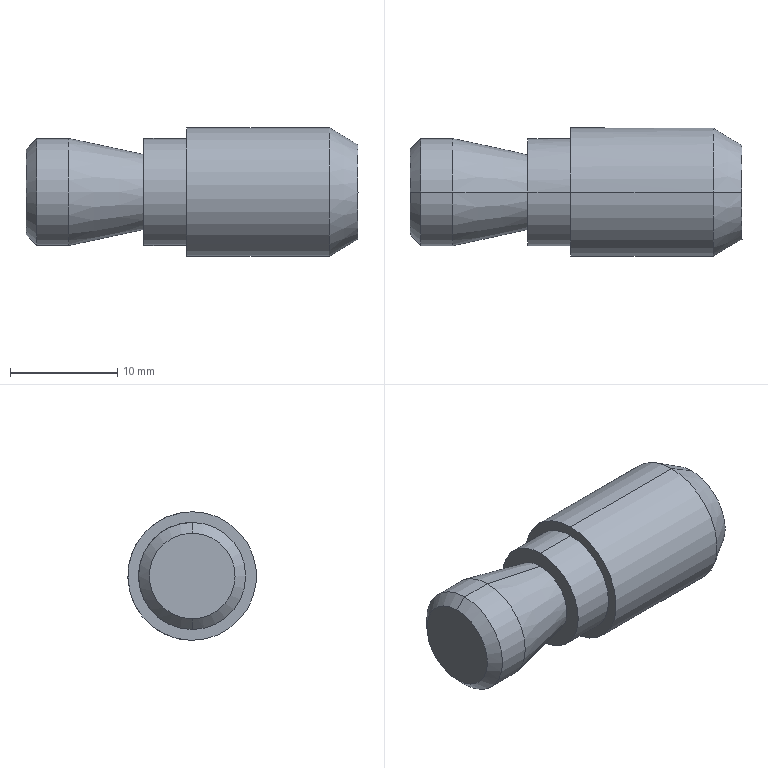Part | STEP file | Positioning_id2322_x_t | 1 solid | 16 faces | box 31 x 12 x 12 mm | volume 2751 mm3 | cone 6 | cylinder 6 | plane 4 | commonest cylinder face diameters 10 x4 12 x2
STEP:
#1=CARTESIAN_POINT('',(0.,0.,0.));
#2=DIRECTION('',(0.,0.,1.));
#3=DIRECTION('',(1.,0.,0.));
#4=AXIS2_PLACEMENT_3D('',#1,#2,#3);
#5=CARTESIAN_POINT('',(-648.,468.,127.399));
#6=VERTEX_POINT('',#5);
#7=CARTESIAN_POINT('',(-650.667,468.,128.999));
#8=VERTEX_POINT('',#7);
#9=CARTESIAN_POINT('',(-648.,468.,127.399));
#10=DIRECTION('',(-0.8575,0.,0.5145));
#11=VECTOR('',#10,1.);
#12=LINE('',#9,#11);
#13=CARTESIAN_POINT('',(-654.,468.,122.999));
#14=DIRECTION('',(-1.,0.,0.));
#15=DIRECTION('',(0.,0.,1.));
#16=AXIS2_PLACEMENT_3D('',#13,#14,#15);
#17=CONICAL_SURFACE('',#16,8.,0.5404);
#18=CARTESIAN_POINT('',(0.,-6.));
#19=DIRECTION('',(0.,1.));
#20=VECTOR('',#19,1.);
#21=LINE('',#18,#20);
#22=(GEOMETRIC_REPRESENTATION_CONTEXT(2)PARAMETRIC_REPRESENTATION_CONTEXT()REPRESENTATION_CONTEXT('',''));
#23=DEFINITIONAL_REPRESENTATION('',(#21),#22);
#24=PCURVE('',#17,#23);
#25=CARTESIAN_POINT('',(-654.,468.,122.999));
#26=DIRECTION('',(-1.,0.,0.));
#27=DIRECTION('',(0.,0.,1.));
#28=AXIS2_PLACEMENT_3D('',#25,#26,#27);
#29=CONICAL_SURFACE('',#28,8.,0.5404);
#30=CARTESIAN_POINT('',(6.283,-6.));
#31=DIRECTION('',(0.,1.));
#32=VECTOR('',#31,1.);
#33=LINE('',#30,#32);
#34=(GEOMETRIC_REPRESENTATION_CONTEXT(2)PARAMETRIC_REPRESENTATION_CONTEXT()REPRESENTATION_CONTEXT('',''));
#35=DEFINITIONAL_REPRESENTATION('',(#33),#34);
#36=PCURVE('',#29,#35);
#37=SURFACE_CURVE('',#12,(#24,#36),.PCURVE_S1.);
#38=EDGE_CURVE('',#6,#8,#37,.T.);
#39=ORIENTED_EDGE('',*,*,#38,.F.);
#40=CARTESIAN_POINT('',(-648.,468.,118.599));
#41=VERTEX_POINT('',#40);
#42=CARTESIAN_POINT('',(-648.,468.,122.999));
#43=DIRECTION('',(-1.,0.,0.));
#44=DIRECTION('',(0.,0.,1.));
#45=AXIS2_PLACEMENT_3D('',#42,#43,#44);
#46=CIRCLE('',#45,4.4);
#47=CARTESIAN_POINT('',(0.,-6.));
#48=DIRECTION('',(1.,0.));
#49=VECTOR('',#48,1.);
#50=LINE('',#47,#49);
#51=(GEOMETRIC_REPRESENTATION_CONTEXT(2)PARAMETRIC_REPRESENTATION_CONTEXT()REPRESENTATION_CONTEXT('',''));
#52=DEFINITIONAL_REPRESENTATION('',(#50),#51);
#53=PCURVE('',#17,#52);
#54=CARTESIAN_POINT('',(-648.,468.,122.999));
#55=DIRECTION('',(1.,0.,0.));
#56=DIRECTION('',(0.,0.,1.));
#57=AXIS2_PLACEMENT_3D('',#54,#55,#56);
#58=PLANE('',#57);
#59=CARTESIAN_POINT('',(4.4,0.));
#60=CARTESIAN_POINT('',(4.4,-7.621));
#61=CARTESIAN_POINT('',(-2.2,-3.811));
#62=CARTESIAN_POINT('',(-8.8,0.));
#63=CARTESIAN_POINT('',(-2.2,3.811));
#64=CARTESIAN_POINT('',(4.4,7.621));
#65=CARTESIAN_POINT('',(4.4,0.));
#66=(BOUNDED_CURVE()B_SPLINE_CURVE(2,(#59,#60,#61,#62,#63,#64,#65),.UNSPECIFIED.,.T.,.F.)B_SPLINE_CURVE_WITH_KNOTS((1,2,2,2,2,1),(-2.094,0.,2.094,4.189,6.283,8.378),.UNSPECIFIED.)CURVE()GEOMETRIC_REPRESENTATION_ITEM()RATIONAL_B_SPLINE_CURVE((1.,0.5,1.,0.5,1.,0.5,1.))REPRESENTATION_ITEM(''));
#67=(GEOMETRIC_REPRESENTATION_CONTEXT(2)PARAMETRIC_REPRESENTATION_CONTEXT()REPRESENTATION_CONTEXT('',''));
#68=DEFINITIONAL_REPRESENTATION('',(#66),#67);
#69=PCURVE('',#58,#68);
#70=SURFACE_CURVE('',#46,(#53,#69),.PCURVE_S1.);
#71=EDGE_CURVE('',#6,#41,#70,.T.);
#72=ORIENTED_EDGE('',*,*,#71,.T.);
#73=CARTESIAN_POINT('',(-650.667,468.,116.999));
#74=VERTEX_POINT('',#73);
#75=CARTESIAN_POINT('',(-648.,468.,118.599));
#76=DIRECTION('',(0.8575,0.,0.5145));
#77=VECTOR('',#76,1.);
#78=LINE('',#75,#77);
#79=CARTESIAN_POINT('',(3.142,-6.));
#80=DIRECTION('',(0.,-1.));
#81=VECTOR('',#80,1.);
#82=LINE('',#79,#81);
#83=(GEOMETRIC_REPRESENTATION_CONTEXT(2)PARAMETRIC_REPRESENTATION_CONTEXT()REPRESENTATION_CONTEXT('',''));
#84=DEFINITIONAL_REPRESENTATION('',(#82),#83);
#85=PCURVE('',#17,#84);
#86=CARTESIAN_POINT('',(3.142,-6.));
#87=DIRECTION('',(0.,-1.));
#88=VECTOR('',#87,1.);
#89=LINE('',#86,#88);
#90=(GEOMETRIC_REPRESENTATION_CONTEXT(2)PARAMETRIC_REPRESENTATION_CONTEXT()REPRESENTATION_CONTEXT('',''));
#91=DEFINITIONAL_REPRESENTATION('',(#89),#90);
#92=PCURVE('',#29,#91);
#93=SURFACE_CURVE('',#78,(#85,#92),.PCURVE_S1.);
#94=EDGE_CURVE('',#74,#41,#93,.T.);
#95=ORIENTED_EDGE('',*,*,#94,.F.);
#96=CARTESIAN_POINT('',(-650.667,468.,122.999));
#97=DIRECTION('',(1.,0.,0.));
#98=DIRECTION('',(0.,0.,-1.));
#99=AXIS2_PLACEMENT_3D('',#96,#97,#98);
#100=CIRCLE('',#99,6.);
#101=CARTESIAN_POINT('',(3.142,-3.333));
#102=DIRECTION('',(-1.,0.));
#103=VECTOR('',#102,1.);
#104=LINE('',#101,#103);
#105=(GEOMETRIC_REPRESENTATION_CONTEXT(2)PARAMETRIC_REPRESENTATION_CONTEXT()REPRESENTATION_CONTEXT('',''));
#106=DEFINITIONAL_REPRESENTATION('',(#104),#105);
#107=PCURVE('',#17,#106);
#108=CARTESIAN_POINT('',(-669.,468.,122.999));
#109=DIRECTION('',(-1.,0.,0.));
#110=DIRECTION('',(0.,0.,1.));
#111=AXIS2_PLACEMENT_3D('',#108,#109,#110);
#112=CYLINDRICAL_SURFACE('',#111,6.);
#113=CARTESIAN_POINT('',(3.142,-18.333));
#114=DIRECTION('',(-1.,0.));
#115=VECTOR('',#114,1.);
#116=LINE('',#113,#115);
#117=(GEOMETRIC_REPRESENTATION_CONTEXT(2)PARAMETRIC_REPRESENTATION_CONTEXT()REPRESENTATION_CONTEXT('',''));
#118=DEFINITIONAL_REPRESENTATION('',(#116),#117);
#119=PCURVE('',#112,#118);
#120=SURFACE_CURVE('',#100,(#107,#119),.PCURVE_S1.);
#121=EDGE_CURVE('',#74,#8,#120,.T.);
#122=ORIENTED_EDGE('',*,*,#121,.T.);
#123=EDGE_LOOP('',(#39,#72,#95,#122));
#124=FACE_BOUND('',#123,.T.);
#125=ADVANCED_FACE('',(#124),#17,.T.);
#126=CARTESIAN_POINT('',(-648.,468.,118.599));
#127=CARTESIAN_POINT('',(-648.,463.6,118.599));
#128=CARTESIAN_POINT('',(-648.,461.4,122.999));
#129=CARTESIAN_POINT('',(-648.,463.6,127.399));
#130=CARTESIAN_POINT('',(-648.,468.,127.399));
#131=(BOUNDED_CURVE()B_SPLINE_CURVE(4,(#126,#127,#128,#129,#130),.UNSPECIFIED.,.F.,.F.)B_SPLINE_CURVE_WITH_KNOTS((5,5),(0.,1.),.PIECEWISE_BEZIER_KNOTS.)CURVE()GEOMETRIC_REPRESENTATION_ITEM()RATIONAL_B_SPLINE_CURVE((1.,0.7071,0.6667,0.7071,1.))REPRESENTATION_ITEM(''));
#132=CARTESIAN_POINT('',(-4.4,0.));
#133=CARTESIAN_POINT('',(-4.4,4.4));
#134=CARTESIAN_POINT('',(0.,6.6));
#135=CARTESIAN_POINT('',(4.4,4.4));
#136=CARTESIAN_POINT('',(4.4,0.));
#137=(BOUNDED_CURVE()B_SPLINE_CURVE(4,(#132,#133,#134,#135,#136),.UNSPECIFIED.,.F.,.F.)B_SPLINE_CURVE_WITH_KNOTS((5,5),(0.,1.),.PIECEWISE_BEZIER_KNOTS.)CURVE()GEOMETRIC_REPRESENTATION_ITEM()RATIONAL_B_SPLINE_CURVE((1.,0.7071,0.6667,0.7071,1.))REPRESENTATION_ITEM(''));
#138=(GEOMETRIC_REPRESENTATION_CONTEXT(2)PARAMETRIC_REPRESENTATION_CONTEXT()REPRESENTATION_CONTEXT('',''));
#139=DEFINITIONAL_REPRESENTATION('',(#137),#138);
#140=PCURVE('',#58,#139);
#141=CARTESIAN_POINT('',(3.142,-6.));
#142=CARTESIAN_POINT('',(3.184,-6.));
#143=CARTESIAN_POINT('',(3.271,-6.));
#144=CARTESIAN_POINT('',(3.405,-6.));
#145=CARTESIAN_POINT('',(3.542,-6.));
#146=CARTESIAN_POINT('',(3.681,-6.));
#147=CARTESIAN_POINT('',(3.823,-6.));
#148=CARTESIAN_POINT('',(3.968,-6.));
#149=CARTESIAN_POINT('',(4.114,-6.));
#150=CARTESIAN_POINT('',(4.262,-6.));
#151=CARTESIAN_POINT('',(4.412,-6.));
#152=CARTESIAN_POINT('',(4.562,-6.));
#153=CARTESIAN_POINT('',(4.712,-6.));
#154=CARTESIAN_POINT('',(4.863,-6.));
#155=CARTESIAN_POINT('',(5.013,-6.));
#156=CARTESIAN_POINT('',(5.163,-6.));
#157=CARTESIAN_POINT('',(5.311,-6.));
#158=CARTESIAN_POINT('',(5.457,-6.));
#159=CARTESIAN_POINT('',(5.602,-6.));
#160=CARTESIAN_POINT('',(5.744,-6.));
#161=CARTESIAN_POINT('',(5.883,-6.));
#162=CARTESIAN_POINT('',(6.02,-6.));
#163=CARTESIAN_POINT('',(6.153,-6.));
#164=CARTESIAN_POINT('',(6.24,-6.));
#165=CARTESIAN_POINT('',(6.283,-6.));
#166=B_SPLINE_CURVE_WITH_KNOTS('',3,(#141,#142,#143,#144,#145,#146,#147,#148,#149,#150,#151,#152,#153,#154,#155,#156,#157,#158,#159,#160,#161,#162,#163,#164,#165),.UNSPECIFIED.,.F.,.F.,(4,1,1,1,1,1,1,1,1,1,1,1,1,1,1,1,1,1,1,1,1,1,4),(0.,0.04545,0.09091,0.1364,0.1818,0.2273,0.2727,0.3182,0.3636,0.4091,0.4545,0.5,0.5455,0.5909,0.6364,0.6818,0.7273,0.7727,0.8182,0.8636,0.9091,0.9545,1.),.QUASI_UNIFORM_KNOTS.);
#167=(GEOMETRIC_REPRESENTATION_CONTEXT(2)PARAMETRIC_REPRESENTATION_CONTEXT()REPRESENTATION_CONTEXT('',''));
#168=DEFINITIONAL_REPRESENTATION('',(#166),#167);
#169=PCURVE('',#29,#168);
#170=SURFACE_CURVE('',#131,(#140,#169),.PCURVE_S1.);
#171=EDGE_CURVE('',#41,#6,#170,.T.);
#172=ORIENTED_EDGE('',*,*,#171,.F.);
#173=ORIENTED_EDGE('',*,*,#71,.F.);
#174=EDGE_LOOP('',(#172,#173));
#175=FACE_BOUND('',#174,.T.);
#176=ADVANCED_FACE('',(#175),#58,.T.);
#177=CARTESIAN_POINT('',(-668.,468.,119.499));
#178=VERTEX_POINT('',#177);
#179=CARTESIAN_POINT('',(-668.,468.,126.499));
#180=VERTEX_POINT('',#179);
#181=CARTESIAN_POINT('',(-668.,468.,122.999));
#182=DIRECTION('',(-1.,0.,0.));
#183=DIRECTION('',(0.,0.,-1.));
#184=AXIS2_PLACEMENT_3D('',#181,#182,#183);
#185=CIRCLE('',#184,3.5);
#186=CARTESIAN_POINT('',(-668.,468.,122.999));
#187=DIRECTION('',(1.,0.,0.));
#188=DIRECTION('',(0.,0.,1.));
#189=AXIS2_PLACEMENT_3D('',#186,#187,#188);
#190=PLANE('',#189);
#191=CARTESIAN_POINT('',(-3.5,0.));
#192=CARTESIAN_POINT('',(-3.5,6.062));
#193=CARTESIAN_POINT('',(1.75,3.031));
#194=CARTESIAN_POINT('',(7.,0.));
#195=CARTESIAN_POINT('',(1.75,-3.031));
#196=CARTESIAN_POINT('',(-3.5,-6.062));
#197=CARTESIAN_POINT('',(-3.5,0.));
#198=(BOUNDED_CURVE()B_SPLINE_CURVE(2,(#191,#192,#193,#194,#195,#196,#197),.UNSPECIFIED.,.T.,.F.)B_SPLINE_CURVE_WITH_KNOTS((1,2,2,2,2,1),(-2.094,0.,2.094,4.189,6.283,8.378),.UNSPECIFIED.)CURVE()GEOMETRIC_REPRESENTATION_ITEM()RATIONAL_B_SPLINE_CURVE((1.,0.5,1.,0.5,1.,0.5,1.))REPRESENTATION_ITEM(''));
#199=(GEOMETRIC_REPRESENTATION_CONTEXT(2)PARAMETRIC_REPRESENTATION_CONTEXT()REPRESENTATION_CONTEXT('',''));
#200=DEFINITIONAL_REPRESENTATION('',(#198),#199);
#201=PCURVE('',#190,#200);
#202=CARTESIAN_POINT('',(-675.,468.,122.999));
#203=DIRECTION('',(-1.,0.,0.));
#204=DIRECTION('',(0.,0.,1.));
#205=AXIS2_PLACEMENT_3D('',#202,#203,#204);
#206=CONICAL_SURFACE('',#205,5.,0.2111);
#207=CARTESIAN_POINT('',(3.142,-7.));
#208=DIRECTION('',(1.,0.));
#209=VECTOR('',#208,1.);
#210=LINE('',#207,#209);
#211=(GEOMETRIC_REPRESENTATION_CONTEXT(2)PARAMETRIC_REPRESENTATION_CONTEXT()REPRESENTATION_CONTEXT('',''));
#212=DEFINITIONAL_REPRESENTATION('',(#210),#211);
#213=PCURVE('',#206,#212);
#214=SURFACE_CURVE('',#185,(#201,#213),.PCURVE_S1.);
#215=EDGE_CURVE('',#178,#180,#214,.T.);
#216=ORIENTED_EDGE('',*,*,#215,.F.);
#217=CARTESIAN_POINT('',(-668.,468.,122.999));
#218=DIRECTION('',(-1.,0.,0.));
#219=DIRECTION('',(0.,0.,1.));
#220=AXIS2_PLACEMENT_3D('',#217,#218,#219);
#221=CIRCLE('',#220,3.5);
#222=CARTESIAN_POINT('',(3.5,0.));
#223=CARTESIAN_POINT('',(3.5,-6.062));
#224=CARTESIAN_POINT('',(-1.75,-3.031));
#225=CARTESIAN_POINT('',(-7.,0.));
#226=CARTESIAN_POINT('',(-1.75,3.031));
#227=CARTESIAN_POINT('',(3.5,6.062));
#228=CARTESIAN_POINT('',(3.5,0.));
#229=(BOUNDED_CURVE()B_SPLINE_CURVE(2,(#222,#223,#224,#225,#226,#227,#228),.UNSPECIFIED.,.T.,.F.)B_SPLINE_CURVE_WITH_KNOTS((1,2,2,2,2,1),(-2.094,0.,2.094,4.189,6.283,8.378),.UNSPECIFIED.)CURVE()GEOMETRIC_REPRESENTATION_ITEM()RATIONAL_B_SPLINE_CURVE((1.,0.5,1.,0.5,1.,0.5,1.))REPRESENTATION_ITEM(''));
#230=(GEOMETRIC_REPRESENTATION_CONTEXT(2)PARAMETRIC_REPRESENTATION_CONTEXT()REPRESENTATION_CONTEXT('',''));
#231=DEFINITIONAL_REPRESENTATION('',(#229),#230);
#232=PCURVE('',#190,#231);
#233=CARTESIAN_POINT('',(-675.,468.,122.999));
#234=DIRECTION('',(-1.,0.,0.));
#235=DIRECTION('',(0.,0.,1.));
#236=AXIS2_PLACEMENT_3D('',#233,#234,#235);
#237=CONICAL_SURFACE('',#236,5.,0.2111);
#238=CARTESIAN_POINT('',(0.,-7.));
#239=DIRECTION('',(1.,0.));
#240=VECTOR('',#239,1.);
#241=LINE('',#238,#240);
#242=(GEOMETRIC_REPRESENTATION_CONTEXT(2)PARAMETRIC_REPRESENTATION_CONTEXT()REPRESENTATION_CONTEXT('',''));
#243=DEFINITIONAL_REPRESENTATION('',(#241),#242);
#244=PCURVE('',#237,#243);
#245=SURFACE_CURVE('',#221,(#232,#244),.PCURVE_S1.);
#246=EDGE_CURVE('',#180,#178,#245,.T.);
#247=ORIENTED_EDGE('',*,*,#246,.F.);
#248=EDGE_LOOP('',(#216,#247));
#249=FACE_BOUND('',#248,.T.);
#250=CARTESIAN_POINT('',(-668.,468.,117.999));
#251=VERTEX_POINT('',#250);
#252=CARTESIAN_POINT('',(-668.,468.,127.999));
#253=VERTEX_POINT('',#252);
#254=CARTESIAN_POINT('',(-668.,468.,122.999));
#255=DIRECTION('',(1.,0.,0.));
#256=DIRECTION('',(0.,0.,-1.));
#257=AXIS2_PLACEMENT_3D('',#254,#255,#256);
#258=CIRCLE('',#257,5.);
#259=CARTESIAN_POINT('',(0.,0.));
#260=DIRECTION('',(-1.,0.));
#261=AXIS2_PLACEMENT_2D('',#259,#260);
#262=CIRCLE('',#261,5.);
#263=(GEOMETRIC_REPRESENTATION_CONTEXT(2)PARAMETRIC_REPRESENTATION_CONTEXT()REPRESENTATION_CONTEXT('',''));
#264=DEFINITIONAL_REPRESENTATION('',(#262),#263);
#265=PCURVE('',#190,#264);
#266=CARTESIAN_POINT('',(-669.,468.,122.999));
#267=DIRECTION('',(-1.,0.,0.));
#268=DIRECTION('',(0.,0.,1.));
#269=AXIS2_PLACEMENT_3D('',#266,#267,#268);
#270=CYLINDRICAL_SURFACE('',#269,5.);
#271=CARTESIAN_POINT('',(3.142,-1.));
#272=DIRECTION('',(-1.,0.));
#273=VECTOR('',#272,1.);
#274=LINE('',#271,#273);
#275=(GEOMETRIC_REPRESENTATION_CONTEXT(2)PARAMETRIC_REPRESENTATION_CONTEXT()REPRESENTATION_CONTEXT('',''));
#276=DEFINITIONAL_REPRESENTATION('',(#274),#275);
#277=PCURVE('',#270,#276);
#278=SURFACE_CURVE('',#258,(#265,#277),.PCURVE_S1.);
#279=EDGE_CURVE('',#251,#253,#278,.T.);
#280=ORIENTED_EDGE('',*,*,#279,.F.);
#281=CARTESIAN_POINT('',(-668.,468.,122.999));
#282=DIRECTION('',(1.,0.,0.));
#283=DIRECTION('',(0.,0.,1.));
#284=AXIS2_PLACEMENT_3D('',#281,#282,#283);
#285=CIRCLE('',#284,5.);
#286=CARTESIAN_POINT('',(0.,0.));
#287=DIRECTION('',(1.,0.));
#288=AXIS2_PLACEMENT_2D('',#286,#287);
#289=CIRCLE('',#288,5.);
#290=(GEOMETRIC_REPRESENTATION_CONTEXT(2)PARAMETRIC_REPRESENTATION_CONTEXT()REPRESENTATION_CONTEXT('',''));
#291=DEFINITIONAL_REPRESENTATION('',(#289),#290);
#292=PCURVE('',#190,#291);
#293=CARTESIAN_POINT('',(-669.,468.,122.999));
#294=DIRECTION('',(-1.,0.,0.));
#295=DIRECTION('',(0.,0.,1.));
#296=AXIS2_PLACEMENT_3D('',#293,#294,#295);
#297=CYLINDRICAL_SURFACE('',#296,5.);
#298=CARTESIAN_POINT('',(6.283,-1.));
#299=DIRECTION('',(-1.,0.));
#300=VECTOR('',#299,1.);
#301=LINE('',#298,#300);
#302=(GEOMETRIC_REPRESENTATION_CONTEXT(2)PARAMETRIC_REPRESENTATION_CONTEXT()REPRESENTATION_CONTEXT('',''));
#303=DEFINITIONAL_REPRESENTATION('',(#301),#302);
#304=PCURVE('',#297,#303);
#305=SURFACE_CURVE('',#285,(#292,#304),.PCURVE_S1.);
#306=EDGE_CURVE('',#253,#251,#305,.T.);
#307=ORIENTED_EDGE('',*,*,#306,.F.);
#308=EDGE_LOOP('',(#280,#307));
#309=FACE_BOUND('',#308,.T.);
#310=ADVANCED_FACE('',(#249,#309),#190,.F.);
#311=CARTESIAN_POINT('',(-664.,468.,127.999));
#312=VERTEX_POINT('',#311);
#313=CARTESIAN_POINT('',(-668.,468.,127.999));
#314=DIRECTION('',(1.,0.,0.));
#315=VECTOR('',#314,1.);
#316=LINE('',#313,#315);
#317=CARTESIAN_POINT('',(6.283,-1.));
#318=DIRECTION('',(0.,-1.));
#319=VECTOR('',#318,1.);
#320=LINE('',#317,#319);
#321=(GEOMETRIC_REPRESENTATION_CONTEXT(2)PARAMETRIC_REPRESENTATION_CONTEXT()REPRESENTATION_CONTEXT('',''));
#322=DEFINITIONAL_REPRESENTATION('',(#320),#321);
#323=PCURVE('',#297,#322);
#324=CARTESIAN_POINT('',(0.,-1.));
#325=DIRECTION('',(0.,-1.));
#326=VECTOR('',#325,1.);
#327=LINE('',#324,#326);
#328=(GEOMETRIC_REPRESENTATION_CONTEXT(2)PARAMETRIC_REPRESENTATION_CONTEXT()REPRESENTATION_CONTEXT('',''));
#329=DEFINITIONAL_REPRESENTATION('',(#327),#328);
#330=PCURVE('',#270,#329);
#331=SURFACE_CURVE('',#316,(#323,#330),.PCURVE_S1.);
#332=EDGE_CURVE('',#253,#312,#331,.T.);
#333=ORIENTED_EDGE('',*,*,#332,.F.);
#334=ORIENTED_EDGE('',*,*,#306,.T.);
#335=CARTESIAN_POINT('',(-664.,468.,117.999));
#336=VERTEX_POINT('',#335);
#337=CARTESIAN_POINT('',(-668.,468.,117.999));
#338=DIRECTION('',(-1.,0.,0.));
#339=VECTOR('',#338,1.);
#340=LINE('',#337,#339);
#341=CARTESIAN_POINT('',(3.142,-1.));
#342=DIRECTION('',(0.,1.));
#343=VECTOR('',#342,1.);
#344=LINE('',#341,#343);
#345=(GEOMETRIC_REPRESENTATION_CONTEXT(2)PARAMETRIC_REPRESENTATION_CONTEXT()REPRESENTATION_CONTEXT('',''));
#346=DEFINITIONAL_REPRESENTATION('',(#344),#345);
#347=PCURVE('',#297,#346);
#348=CARTESIAN_POINT('',(3.142,-1.));
#349=DIRECTION('',(0.,1.));
#350=VECTOR('',#349,1.);
#351=LINE('',#348,#350);
#352=(GEOMETRIC_REPRESENTATION_CONTEXT(2)PARAMETRIC_REPRESENTATION_CONTEXT()REPRESENTATION_CONTEXT('',''));
#353=DEFINITIONAL_REPRESENTATION('',(#351),#352);
#354=PCURVE('',#270,#353);
#355=SURFACE_CURVE('',#340,(#347,#354),.PCURVE_S1.);
#356=EDGE_CURVE('',#336,#251,#355,.T.);
#357=ORIENTED_EDGE('',*,*,#356,.F.);
#358=CARTESIAN_POINT('',(-664.,468.,122.999));
#359=DIRECTION('',(1.,0.,0.));
#360=DIRECTION('',(0.,0.,1.));
#361=AXIS2_PLACEMENT_3D('',#358,#359,#360);
#362=CIRCLE('',#361,5.);
#363=CARTESIAN_POINT('',(6.283,-5.));
#364=DIRECTION('',(-1.,0.));
#365=VECTOR('',#364,1.);
#366=LINE('',#363,#365);
#367=(GEOMETRIC_REPRESENTATION_CONTEXT(2)PARAMETRIC_REPRESENTATION_CONTEXT()REPRESENTATION_CONTEXT('',''));
#368=DEFINITIONAL_REPRESENTATION('',(#366),#367);
#369=PCURVE('',#297,#368);
#370=CARTESIAN_POINT('',(-664.,468.,122.999));
#371=DIRECTION('',(-1.,0.,0.));
#372=DIRECTION('',(0.,0.,-1.));
#373=AXIS2_PLACEMENT_3D('',#370,#371,#372);
#374=PLANE('',#373);
#375=CARTESIAN_POINT('',(-5.,0.));
#376=CARTESIAN_POINT('',(-5.,8.66));
#377=CARTESIAN_POINT('',(2.5,4.33));
#378=CARTESIAN_POINT('',(10.,0.));
#379=CARTESIAN_POINT('',(2.5,-4.33));
#380=CARTESIAN_POINT('',(-5.,-8.66));
#381=CARTESIAN_POINT('',(-5.,0.));
#382=(BOUNDED_CURVE()B_SPLINE_CURVE(2,(#375,#376,#377,#378,#379,#380,#381),.UNSPECIFIED.,.T.,.F.)B_SPLINE_CURVE_WITH_KNOTS((1,2,2,2,2,1),(-2.094,0.,2.094,4.189,6.283,8.378),.UNSPECIFIED.)CURVE()GEOMETRIC_REPRESENTATION_ITEM()RATIONAL_B_SPLINE_CURVE((1.,0.5,1.,0.5,1.,0.5,1.))REPRESENTATION_ITEM(''));
#383=(GEOMETRIC_REPRESENTATION_CONTEXT(2)PARAMETRIC_REPRESENTATION_CONTEXT()REPRESENTATION_CONTEXT('',''));
#384=DEFINITIONAL_REPRESENTATION('',(#382),#383);
#385=PCURVE('',#374,#384);
#386=SURFACE_CURVE('',#362,(#369,#385),.PCURVE_S1.);
#387=EDGE_CURVE('',#312,#336,#386,.T.);
#388=ORIENTED_EDGE('',*,*,#387,.F.);
#389=EDGE_LOOP('',(#333,#334,#357,#388));
#390=FACE_BOUND('',#389,.T.);
#391=ADVANCED_FACE('',(#390),#297,.T.);
#392=CARTESIAN_POINT('',(-675.,468.,127.999));
#393=VERTEX_POINT('',#392);
#394=CARTESIAN_POINT('',(-668.,468.,126.499));
#395=DIRECTION('',(0.9778,0.,-0.2095));
#396=VECTOR('',#395,1.);
#397=LINE('',#394,#396);
#398=CARTESIAN_POINT('',(0.,-7.));
#399=DIRECTION('',(0.,-1.));
#400=VECTOR('',#399,1.);
#401=LINE('',#398,#400);
#402=(GEOMETRIC_REPRESENTATION_CONTEXT(2)PARAMETRIC_REPRESENTATION_CONTEXT()REPRESENTATION_CONTEXT('',''));
#403=DEFINITIONAL_REPRESENTATION('',(#401),#402);
#404=PCURVE('',#237,#403);
#405=CARTESIAN_POINT('',(6.283,-7.));
#406=DIRECTION('',(0.,-1.));
#407=VECTOR('',#406,1.);
#408=LINE('',#405,#407);
#409=(GEOMETRIC_REPRESENTATION_CONTEXT(2)PARAMETRIC_REPRESENTATION_CONTEXT()REPRESENTATION_CONTEXT('',''));
#410=DEFINITIONAL_REPRESENTATION('',(#408),#409);
#411=PCURVE('',#206,#410);
#412=SURFACE_CURVE('',#397,(#404,#411),.PCURVE_S1.);
#413=EDGE_CURVE('',#393,#180,#412,.T.);
#414=ORIENTED_EDGE('',*,*,#413,.T.);
#415=ORIENTED_EDGE('',*,*,#246,.T.);
#416=CARTESIAN_POINT('',(-675.,468.,117.999));
#417=VERTEX_POINT('',#416);
#418=CARTESIAN_POINT('',(-668.,468.,119.499));
#419=DIRECTION('',(-0.9778,0.,-0.2095));
#420=VECTOR('',#419,1.);
#421=LINE('',#418,#420);
#422=CARTESIAN_POINT('',(3.142,-7.));
#423=DIRECTION('',(0.,1.));
#424=VECTOR('',#423,1.);
#425=LINE('',#422,#424);
#426=(GEOMETRIC_REPRESENTATION_CONTEXT(2)PARAMETRIC_REPRESENTATION_CONTEXT()REPRESENTATION_CONTEXT('',''));
#427=DEFINITIONAL_REPRESENTATION('',(#425),#426);
#428=PCURVE('',#237,#427);
#429=CARTESIAN_POINT('',(3.142,-7.));
#430=DIRECTION('',(0.,1.));
#431=VECTOR('',#430,1.);
#432=LINE('',#429,#431);
#433=(GEOMETRIC_REPRESENTATION_CONTEXT(2)PARAMETRIC_REPRESENTATION_CONTEXT()REPRESENTATION_CONTEXT('',''));
#434=DEFINITIONAL_REPRESENTATION('',(#432),#433);
#435=PCURVE('',#206,#434);
#436=SURFACE_CURVE('',#421,(#428,#435),.PCURVE_S1.);
#437=EDGE_CURVE('',#178,#417,#436,.T.);
#438=ORIENTED_EDGE('',*,*,#437,.T.);
#439=CARTESIAN_POINT('',(-675.,468.,122.999));
#440=DIRECTION('',(1.,0.,0.));
#441=DIRECTION('',(0.,0.,-1.));
#442=AXIS2_PLACEMENT_3D('',#439,#440,#441);
#443=CIRCLE('',#442,5.);
#444=CARTESIAN_POINT('',(3.142,0.));
#445=DIRECTION('',(-1.,0.));
#446=VECTOR('',#445,1.);
#447=LINE('',#444,#446);
#448=(GEOMETRIC_REPRESENTATION_CONTEXT(2)PARAMETRIC_REPRESENTATION_CONTEXT()REPRESENTATION_CONTEXT('',''));
#449=DEFINITIONAL_REPRESENTATION('',(#447),#448);
#450=PCURVE('',#237,#449);
#451=CARTESIAN_POINT('',(-669.,468.,122.999));
#452=DIRECTION('',(-1.,0.,0.));
#453=DIRECTION('',(0.,0.,1.));
#454=AXIS2_PLACEMENT_3D('',#451,#452,#453);
#455=CYLINDRICAL_SURFACE('',#454,5.);
#456=CARTESIAN_POINT('',(3.142,6.));
#457=DIRECTION('',(-1.,0.));
#458=VECTOR('',#457,1.);
#459=LINE('',#456,#458);
#460=(GEOMETRIC_REPRESENTATION_CONTEXT(2)PARAMETRIC_REPRESENTATION_CONTEXT()REPRESENTATION_CONTEXT('',''));
#461=DEFINITIONAL_REPRESENTATION('',(#459),#460);
#462=PCURVE('',#455,#461);
#463=SURFACE_CURVE('',#443,(#450,#462),.PCURVE_S1.);
#464=EDGE_CURVE('',#417,#393,#463,.T.);
#465=ORIENTED_EDGE('',*,*,#464,.T.);
#466=EDGE_LOOP('',(#414,#415,#438,#465));
#467=FACE_BOUND('',#466,.T.);
#468=ADVANCED_FACE('',(#467),#237,.T.);
#469=CARTESIAN_POINT('',(-678.,468.,117.999));
#470=VERTEX_POINT('',#469);
#471=CARTESIAN_POINT('',(-679.,468.,118.999));
#472=VERTEX_POINT('',#471);
#473=CARTESIAN_POINT('',(-679.,468.,118.999));
#474=DIRECTION('',(-0.7071,0.,0.7071));
#475=VECTOR('',#474,1.);
#476=LINE('',#473,#475);
#477=CARTESIAN_POINT('',(-678.,468.,122.999));
#478=DIRECTION('',(1.,0.,0.));
#479=DIRECTION('',(0.,0.,-1.));
#480=AXIS2_PLACEMENT_3D('',#477,#478,#479);
#481=CONICAL_SURFACE('',#480,5.,0.7854);
#482=CARTESIAN_POINT('',(0.,-1.));
#483=DIRECTION('',(0.,-1.));
#484=VECTOR('',#483,1.);
#485=LINE('',#482,#484);
#486=(GEOMETRIC_REPRESENTATION_CONTEXT(2)PARAMETRIC_REPRESENTATION_CONTEXT()REPRESENTATION_CONTEXT('',''));
#487=DEFINITIONAL_REPRESENTATION('',(#485),#486);
#488=PCURVE('',#481,#487);
#489=CARTESIAN_POINT('',(-678.,468.,122.999));
#490=DIRECTION('',(1.,0.,0.));
#491=DIRECTION('',(0.,0.,-1.));
#492=AXIS2_PLACEMENT_3D('',#489,#490,#491);
#493=CONICAL_SURFACE('',#492,5.,0.7854);
#494=CARTESIAN_POINT('',(6.283,-1.));
#495=DIRECTION('',(0.,-1.));
#496=VECTOR('',#495,1.);
#497=LINE('',#494,#496);
#498=(GEOMETRIC_REPRESENTATION_CONTEXT(2)PARAMETRIC_REPRESENTATION_CONTEXT()REPRESENTATION_CONTEXT('',''));
#499=DEFINITIONAL_REPRESENTATION('',(#497),#498);
#500=PCURVE('',#493,#499);
#501=SURFACE_CURVE('',#476,(#488,#500),.PCURVE_S1.);
#502=EDGE_CURVE('',#470,#472,#501,.T.);
#503=ORIENTED_EDGE('',*,*,#502,.T.);
#504=CARTESIAN_POINT('',(-679.,468.,126.999));
#505=VERTEX_POINT('',#504);
#506=CARTESIAN_POINT('',(-679.,468.,122.999));
#507=DIRECTION('',(1.,0.,0.));
#508=DIRECTION('',(0.,0.,-1.));
#509=AXIS2_PLACEMENT_3D('',#506,#507,#508);
#510=CIRCLE('',#509,4.);
#511=CARTESIAN_POINT('',(0.,-1.));
#512=DIRECTION('',(1.,0.));
#513=VECTOR('',#512,1.);
#514=LINE('',#511,#513);
#515=(GEOMETRIC_REPRESENTATION_CONTEXT(2)PARAMETRIC_REPRESENTATION_CONTEXT()REPRESENTATION_CONTEXT('',''));
#516=DEFINITIONAL_REPRESENTATION('',(#514),#515);
#517=PCURVE('',#481,#516);
#518=CARTESIAN_POINT('',(-679.,468.,122.999));
#519=DIRECTION('',(-1.,0.,0.));
#520=DIRECTION('',(0.,0.,-1.));
#521=AXIS2_PLACEMENT_3D('',#518,#519,#520);
#522=PLANE('',#521);
#523=CARTESIAN_POINT('',(4.,0.));
#524=CARTESIAN_POINT('',(4.,-6.928));
#525=CARTESIAN_POINT('',(-2.,-3.464));
#526=CARTESIAN_POINT('',(-8.,0.));
#527=CARTESIAN_POINT('',(-2.,3.464));
#528=CARTESIAN_POINT('',(4.,6.928));
#529=CARTESIAN_POINT('',(4.,0.));
#530=(BOUNDED_CURVE()B_SPLINE_CURVE(2,(#523,#524,#525,#526,#527,#528,#529),.UNSPECIFIED.,.T.,.F.)B_SPLINE_CURVE_WITH_KNOTS((1,2,2,2,2,1),(-2.094,0.,2.094,4.189,6.283,8.378),.UNSPECIFIED.)CURVE()GEOMETRIC_REPRESENTATION_ITEM()RATIONAL_B_SPLINE_CURVE((1.,0.5,1.,0.5,1.,0.5,1.))REPRESENTATION_ITEM(''));
#531=(GEOMETRIC_REPRESENTATION_CONTEXT(2)PARAMETRIC_REPRESENTATION_CONTEXT()REPRESENTATION_CONTEXT('',''));
#532=DEFINITIONAL_REPRESENTATION('',(#530),#531);
#533=PCURVE('',#522,#532);
#534=SURFACE_CURVE('',#510,(#517,#533),.PCURVE_S1.);
#535=EDGE_CURVE('',#472,#505,#534,.T.);
#536=ORIENTED_EDGE('',*,*,#535,.T.);
#537=CARTESIAN_POINT('',(-678.,468.,127.999));
#538=VERTEX_POINT('',#537);
#539=CARTESIAN_POINT('',(-679.,468.,126.999));
#540=DIRECTION('',(0.7071,0.,0.7071));
#541=VECTOR('',#540,1.);
#542=LINE('',#539,#541);
#543=CARTESIAN_POINT('',(3.142,-1.));
#544=DIRECTION('',(0.,1.));
#545=VECTOR('',#544,1.);
#546=LINE('',#543,#545);
#547=(GEOMETRIC_REPRESENTATION_CONTEXT(2)PARAMETRIC_REPRESENTATION_CONTEXT()REPRESENTATION_CONTEXT('',''));
#548=DEFINITIONAL_REPRESENTATION('',(#546),#547);
#549=PCURVE('',#481,#548);
#550=CARTESIAN_POINT('',(3.142,-1.));
#551=DIRECTION('',(0.,1.));
#552=VECTOR('',#551,1.);
#553=LINE('',#550,#552);
#554=(GEOMETRIC_REPRESENTATION_CONTEXT(2)PARAMETRIC_REPRESENTATION_CONTEXT()REPRESENTATION_CONTEXT('',''));
#555=DEFINITIONAL_REPRESENTATION('',(#553),#554);
#556=PCURVE('',#493,#555);
#557=SURFACE_CURVE('',#542,(#549,#556),.PCURVE_S1.);
#558=EDGE_CURVE('',#505,#538,#557,.T.);
#559=ORIENTED_EDGE('',*,*,#558,.T.);
#560=CARTESIAN_POINT('',(-678.,468.,122.999));
#561=DIRECTION('',(-1.,0.,0.));
#562=DIRECTION('',(0.,0.,1.));
#563=AXIS2_PLACEMENT_3D('',#560,#561,#562);
#564=CIRCLE('',#563,5.);
#565=CARTESIAN_POINT('',(3.142,0.));
#566=DIRECTION('',(-1.,0.));
#567=VECTOR('',#566,1.);
#568=LINE('',#565,#567);
#569=(GEOMETRIC_REPRESENTATION_CONTEXT(2)PARAMETRIC_REPRESENTATION_CONTEXT()REPRESENTATION_CONTEXT('',''));
#570=DEFINITIONAL_REPRESENTATION('',(#568),#569);
#571=PCURVE('',#481,#570);
#572=CARTESIAN_POINT('',(0.,9.));
#573=DIRECTION('',(1.,0.));
#574=VECTOR('',#573,1.);
#575=LINE('',#572,#574);
#576=(GEOMETRIC_REPRESENTATION_CONTEXT(2)PARAMETRIC_REPRESENTATION_CONTEXT()REPRESENTATION_CONTEXT('',''));
#577=DEFINITIONAL_REPRESENTATION('',(#575),#576);
#578=PCURVE('',#455,#577);
#579=SURFACE_CURVE('',#564,(#571,#578),.PCURVE_S1.);
#580=EDGE_CURVE('',#538,#470,#579,.T.);
#581=ORIENTED_EDGE('',*,*,#580,.T.);
#582=EDGE_LOOP('',(#503,#536,#559,#581));
#583=FACE_BOUND('',#582,.T.);
#584=ADVANCED_FACE('',(#583),#481,.T.);
#585=CARTESIAN_POINT('',(-678.,468.,127.999));
#586=DIRECTION('',(-1.,0.,0.));
#587=VECTOR('',#586,1.);
#588=LINE('',#585,#587);
#589=CARTESIAN_POINT('',(-669.,468.,122.999));
#590=DIRECTION('',(-1.,0.,0.));
#591=DIRECTION('',(0.,0.,1.));
#592=AXIS2_PLACEMENT_3D('',#589,#590,#591);
#593=CYLINDRICAL_SURFACE('',#592,5.);
#594=CARTESIAN_POINT('',(6.283,9.));
#595=DIRECTION('',(0.,1.));
#596=VECTOR('',#595,1.);
#597=LINE('',#594,#596);
#598=(GEOMETRIC_REPRESENTATION_CONTEXT(2)PARAMETRIC_REPRESENTATION_CONTEXT()REPRESENTATION_CONTEXT('',''));
#599=DEFINITIONAL_REPRESENTATION('',(#597),#598);
#600=PCURVE('',#593,#599);
#601=CARTESIAN_POINT('',(0.,9.));
#602=DIRECTION('',(0.,1.));
#603=VECTOR('',#602,1.);
#604=LINE('',#601,#603);
#605=(GEOMETRIC_REPRESENTATION_CONTEXT(2)PARAMETRIC_REPRESENTATION_CONTEXT()REPRESENTATION_CONTEXT('',''));
#606=DEFINITIONAL_REPRESENTATION('',(#604),#605);
#607=PCURVE('',#455,#606);
#608=SURFACE_CURVE('',#588,(#600,#607),.PCURVE_S1.);
#609=EDGE_CURVE('',#393,#538,#608,.T.);
#610=ORIENTED_EDGE('',*,*,#609,.T.);
#611=CARTESIAN_POINT('',(-678.,468.,122.999));
#612=DIRECTION('',(-1.,0.,0.));
#613=DIRECTION('',(0.,0.,-1.));
#614=AXIS2_PLACEMENT_3D('',#611,#612,#613);
#615=CIRCLE('',#614,5.);
#616=CARTESIAN_POINT('',(3.142,9.));
#617=DIRECTION('',(1.,0.));
#618=VECTOR('',#617,1.);
#619=LINE('',#616,#618);
#620=(GEOMETRIC_REPRESENTATION_CONTEXT(2)PARAMETRIC_REPRESENTATION_CONTEXT()REPRESENTATION_CONTEXT('',''));
#621=DEFINITIONAL_REPRESENTATION('',(#619),#620);
#622=PCURVE('',#593,#621);
#623=CARTESIAN_POINT('',(6.283,0.));
#624=DIRECTION('',(-1.,0.));
#625=VECTOR('',#624,1.);
#626=LINE('',#623,#625);
#627=(GEOMETRIC_REPRESENTATION_CONTEXT(2)PARAMETRIC_REPRESENTATION_CONTEXT()REPRESENTATION_CONTEXT('',''));
#628=DEFINITIONAL_REPRESENTATION('',(#626),#627);
#629=PCURVE('',#493,#628);
#630=SURFACE_CURVE('',#615,(#622,#629),.PCURVE_S1.);
#631=EDGE_CURVE('',#470,#538,#630,.T.);
#632=ORIENTED_EDGE('',*,*,#631,.F.);
#633=CARTESIAN_POINT('',(-678.,468.,117.999));
#634=DIRECTION('',(1.,0.,0.));
#635=VECTOR('',#634,1.);
#636=LINE('',#633,#635);
#637=CARTESIAN_POINT('',(3.142,9.));
#638=DIRECTION('',(0.,-1.));
#639=VECTOR('',#638,1.);
#640=LINE('',#637,#639);
#641=(GEOMETRIC_REPRESENTATION_CONTEXT(2)PARAMETRIC_REPRESENTATION_CONTEXT()REPRESENTATION_CONTEXT('',''));
#642=DEFINITIONAL_REPRESENTATION('',(#640),#641);
#643=PCURVE('',#593,#642);
#644=CARTESIAN_POINT('',(3.142,9.));
#645=DIRECTION('',(0.,-1.));
#646=VECTOR('',#645,1.);
#647=LINE('',#644,#646);
#648=(GEOMETRIC_REPRESENTATION_CONTEXT(2)PARAMETRIC_REPRESENTATION_CONTEXT()REPRESENTATION_CONTEXT('',''));
#649=DEFINITIONAL_REPRESENTATION('',(#647),#648);
#650=PCURVE('',#455,#649);
#651=SURFACE_CURVE('',#636,(#643,#650),.PCURVE_S1.);
#652=EDGE_CURVE('',#470,#417,#651,.T.);
#653=ORIENTED_EDGE('',*,*,#652,.T.);
#654=CARTESIAN_POINT('',(-675.,468.,122.999));
#655=DIRECTION('',(1.,0.,0.));
#656=DIRECTION('',(0.,0.,1.));
#657=AXIS2_PLACEMENT_3D('',#654,#655,#656);
#658=CIRCLE('',#657,5.);
#659=CARTESIAN_POINT('',(6.283,6.));
#660=DIRECTION('',(-1.,0.));
#661=VECTOR('',#660,1.);
#662=LINE('',#659,#661);
#663=(GEOMETRIC_REPRESENTATION_CONTEXT(2)PARAMETRIC_REPRESENTATION_CONTEXT()REPRESENTATION_CONTEXT('',''));
#664=DEFINITIONAL_REPRESENTATION('',(#662),#663);
#665=PCURVE('',#593,#664);
#666=CARTESIAN_POINT('',(6.283,0.));
#667=DIRECTION('',(-1.,0.));
#668=VECTOR('',#667,1.);
#669=LINE('',#666,#668);
#670=(GEOMETRIC_REPRESENTATION_CONTEXT(2)PARAMETRIC_REPRESENTATION_CONTEXT()REPRESENTATION_CONTEXT('',''));
#671=DEFINITIONAL_REPRESENTATION('',(#669),#670);
#672=PCURVE('',#206,#671);
#673=SURFACE_CURVE('',#658,(#665,#672),.PCURVE_S1.);
#674=EDGE_CURVE('',#393,#417,#673,.T.);
#675=ORIENTED_EDGE('',*,*,#674,.F.);
#676=EDGE_LOOP('',(#610,#632,#653,#675));
#677=FACE_BOUND('',#676,.T.);
#678=ADVANCED_FACE('',(#677),#593,.T.);
#679=CARTESIAN_POINT('',(-679.,468.,126.999));
#680=CARTESIAN_POINT('',(-679.,464.,126.999));
#681=CARTESIAN_POINT('',(-679.,462.,122.999));
#682=CARTESIAN_POINT('',(-679.,464.,118.999));
#683=CARTESIAN_POINT('',(-679.,468.,118.999));
#684=(BOUNDED_CURVE()B_SPLINE_CURVE(4,(#679,#680,#681,#682,#683),.UNSPECIFIED.,.F.,.F.)B_SPLINE_CURVE_WITH_KNOTS((5,5),(0.,1.),.PIECEWISE_BEZIER_KNOTS.)CURVE()GEOMETRIC_REPRESENTATION_ITEM()RATIONAL_B_SPLINE_CURVE((1.,0.7071,0.6667,0.7071,1.))REPRESENTATION_ITEM(''));
#685=CARTESIAN_POINT('',(-4.,0.));
#686=CARTESIAN_POINT('',(-4.,4.));
#687=CARTESIAN_POINT('',(0.,6.));
#688=CARTESIAN_POINT('',(4.,4.));
#689=CARTESIAN_POINT('',(4.,0.));
#690=(BOUNDED_CURVE()B_SPLINE_CURVE(4,(#685,#686,#687,#688,#689),.UNSPECIFIED.,.F.,.F.)B_SPLINE_CURVE_WITH_KNOTS((5,5),(0.,1.),.PIECEWISE_BEZIER_KNOTS.)CURVE()GEOMETRIC_REPRESENTATION_ITEM()RATIONAL_B_SPLINE_CURVE((1.,0.7071,0.6667,0.7071,1.))REPRESENTATION_ITEM(''));
#691=(GEOMETRIC_REPRESENTATION_CONTEXT(2)PARAMETRIC_REPRESENTATION_CONTEXT()REPRESENTATION_CONTEXT('',''));
#692=DEFINITIONAL_REPRESENTATION('',(#690),#691);
#693=PCURVE('',#522,#692);
#694=CARTESIAN_POINT('',(3.142,-1.));
#695=CARTESIAN_POINT('',(3.184,-1.));
#696=CARTESIAN_POINT('',(3.271,-1.));
#697=CARTESIAN_POINT('',(3.405,-1.));
#698=CARTESIAN_POINT('',(3.542,-1.));
#699=CARTESIAN_POINT('',(3.681,-1.));
#700=CARTESIAN_POINT('',(3.823,-1.));
#701=CARTESIAN_POINT('',(3.968,-1.));
#702=CARTESIAN_POINT('',(4.114,-1.));
#703=CARTESIAN_POINT('',(4.262,-1.));
#704=CARTESIAN_POINT('',(4.412,-1.));
#705=CARTESIAN_POINT('',(4.562,-1.));
#706=CARTESIAN_POINT('',(4.712,-1.));
#707=CARTESIAN_POINT('',(4.863,-1.));
#708=CARTESIAN_POINT('',(5.013,-1.));
#709=CARTESIAN_POINT('',(5.163,-1.));
#710=CARTESIAN_POINT('',(5.311,-1.));
#711=CARTESIAN_POINT('',(5.457,-1.));
#712=CARTESIAN_POINT('',(5.602,-1.));
#713=CARTESIAN_POINT('',(5.744,-1.));
#714=CARTESIAN_POINT('',(5.883,-1.));
#715=CARTESIAN_POINT('',(6.02,-1.));
#716=CARTESIAN_POINT('',(6.153,-1.));
#717=CARTESIAN_POINT('',(6.24,-1.));
#718=CARTESIAN_POINT('',(6.283,-1.));
#719=B_SPLINE_CURVE_WITH_KNOTS('',3,(#694,#695,#696,#697,#698,#699,#700,#701,#702,#703,#704,#705,#706,#707,#708,#709,#710,#711,#712,#713,#714,#715,#716,#717,#718),.UNSPECIFIED.,.F.,.F.,(4,1,1,1,1,1,1,1,1,1,1,1,1,1,1,1,1,1,1,1,1,1,4),(0.,0.04545,0.09091,0.1364,0.1818,0.2273,0.2727,0.3182,0.3636,0.4091,0.4545,0.5,0.5455,0.5909,0.6364,0.6818,0.7273,0.7727,0.8182,0.8636,0.9091,0.9545,1.),.QUASI_UNIFORM_KNOTS.);
#720=(GEOMETRIC_REPRESENTATION_CONTEXT(2)PARAMETRIC_REPRESENTATION_CONTEXT()REPRESENTATION_CONTEXT('',''));
#721=DEFINITIONAL_REPRESENTATION('',(#719),#720);
#722=PCURVE('',#493,#721);
#723=SURFACE_CURVE('',#684,(#693,#722),.PCURVE_S1.);
#724=EDGE_CURVE('',#505,#472,#723,.T.);
#725=ORIENTED_EDGE('',*,*,#724,.F.);
#726=ORIENTED_EDGE('',*,*,#535,.F.);
#727=EDGE_LOOP('',(#725,#726));
#728=FACE_BOUND('',#727,.T.);
#729=ADVANCED_FACE('',(#728),#522,.T.);
#730=CARTESIAN_POINT('',(-664.,468.,128.999));
#731=VERTEX_POINT('',#730);
#732=CARTESIAN_POINT('',(-664.,468.,128.999));
#733=DIRECTION('',(-1.,0.,0.));
#734=VECTOR('',#733,1.);
#735=LINE('',#732,#734);
#736=CARTESIAN_POINT('',(-669.,468.,122.999));
#737=DIRECTION('',(-1.,0.,0.));
#738=DIRECTION('',(0.,0.,1.));
#739=AXIS2_PLACEMENT_3D('',#736,#737,#738);
#740=CYLINDRICAL_SURFACE('',#739,6.);
#741=CARTESIAN_POINT('',(6.283,-5.));
#742=DIRECTION('',(0.,1.));
#743=VECTOR('',#742,1.);
#744=LINE('',#741,#743);
#745=(GEOMETRIC_REPRESENTATION_CONTEXT(2)PARAMETRIC_REPRESENTATION_CONTEXT()REPRESENTATION_CONTEXT('',''));
#746=DEFINITIONAL_REPRESENTATION('',(#744),#745);
#747=PCURVE('',#740,#746);
#748=CARTESIAN_POINT('',(0.,-5.));
#749=DIRECTION('',(0.,1.));
#750=VECTOR('',#749,1.);
#751=LINE('',#748,#750);
#752=(GEOMETRIC_REPRESENTATION_CONTEXT(2)PARAMETRIC_REPRESENTATION_CONTEXT()REPRESENTATION_CONTEXT('',''));
#753=DEFINITIONAL_REPRESENTATION('',(#751),#752);
#754=PCURVE('',#112,#753);
#755=SURFACE_CURVE('',#735,(#747,#754),.PCURVE_S1.);
#756=EDGE_CURVE('',#8,#731,#755,.T.);
#757=ORIENTED_EDGE('',*,*,#756,.T.);
#758=CARTESIAN_POINT('',(-664.,468.,116.999));
#759=VERTEX_POINT('',#758);
#760=CARTESIAN_POINT('',(-664.,468.,122.999));
#761=DIRECTION('',(-1.,0.,0.));
#762=DIRECTION('',(0.,0.,1.));
#763=AXIS2_PLACEMENT_3D('',#760,#761,#762);
#764=CIRCLE('',#763,6.);
#765=CARTESIAN_POINT('',(0.,-5.));
#766=DIRECTION('',(1.,0.));
#767=VECTOR('',#766,1.);
#768=LINE('',#765,#767);
#769=(GEOMETRIC_REPRESENTATION_CONTEXT(2)PARAMETRIC_REPRESENTATION_CONTEXT()REPRESENTATION_CONTEXT('',''));
#770=DEFINITIONAL_REPRESENTATION('',(#768),#769);
#771=PCURVE('',#740,#770);
#772=CARTESIAN_POINT('',(0.,0.));
#773=DIRECTION('',(-1.,0.));
#774=AXIS2_PLACEMENT_2D('',#772,#773);
#775=CIRCLE('',#774,6.);
#776=(GEOMETRIC_REPRESENTATION_CONTEXT(2)PARAMETRIC_REPRESENTATION_CONTEXT()REPRESENTATION_CONTEXT('',''));
#777=DEFINITIONAL_REPRESENTATION('',(#775),#776);
#778=PCURVE('',#374,#777);
#779=SURFACE_CURVE('',#764,(#771,#778),.PCURVE_S1.);
#780=EDGE_CURVE('',#759,#731,#779,.T.);
#781=ORIENTED_EDGE('',*,*,#780,.F.);
#782=CARTESIAN_POINT('',(-664.,468.,116.999));
#783=DIRECTION('',(1.,0.,0.));
#784=VECTOR('',#783,1.);
#785=LINE('',#782,#784);
#786=CARTESIAN_POINT('',(3.142,-5.));
#787=DIRECTION('',(0.,-1.));
#788=VECTOR('',#787,1.);
#789=LINE('',#786,#788);
#790=(GEOMETRIC_REPRESENTATION_CONTEXT(2)PARAMETRIC_REPRESENTATION_CONTEXT()REPRESENTATION_CONTEXT('',''));
#791=DEFINITIONAL_REPRESENTATION('',(#789),#790);
#792=PCURVE('',#740,#791);
#793=CARTESIAN_POINT('',(3.142,-5.));
#794=DIRECTION('',(0.,-1.));
#795=VECTOR('',#794,1.);
#796=LINE('',#793,#795);
#797=(GEOMETRIC_REPRESENTATION_CONTEXT(2)PARAMETRIC_REPRESENTATION_CONTEXT()REPRESENTATION_CONTEXT('',''));
#798=DEFINITIONAL_REPRESENTATION('',(#796),#797);
#799=PCURVE('',#112,#798);
#800=SURFACE_CURVE('',#785,(#792,#799),.PCURVE_S1.);
#801=EDGE_CURVE('',#759,#74,#800,.T.);
#802=ORIENTED_EDGE('',*,*,#801,.T.);
#803=CARTESIAN_POINT('',(-650.667,468.,122.999));
#804=DIRECTION('',(1.,0.,0.));
#805=DIRECTION('',(0.,0.,1.));
#806=AXIS2_PLACEMENT_3D('',#803,#804,#805);
#807=CIRCLE('',#806,6.);
#808=CARTESIAN_POINT('',(6.283,-18.333));
#809=DIRECTION('',(-1.,0.));
#810=VECTOR('',#809,1.);
#811=LINE('',#808,#810);
#812=(GEOMETRIC_REPRESENTATION_CONTEXT(2)PARAMETRIC_REPRESENTATION_CONTEXT()REPRESENTATION_CONTEXT('',''));
#813=DEFINITIONAL_REPRESENTATION('',(#811),#812);
#814=PCURVE('',#740,#813);
#815=CARTESIAN_POINT('',(6.283,-3.333));
#816=DIRECTION('',(-1.,0.));
#817=VECTOR('',#816,1.);
#818=LINE('',#815,#817);
#819=(GEOMETRIC_REPRESENTATION_CONTEXT(2)PARAMETRIC_REPRESENTATION_CONTEXT()REPRESENTATION_CONTEXT('',''));
#820=DEFINITIONAL_REPRESENTATION('',(#818),#819);
#821=PCURVE('',#29,#820);
#822=SURFACE_CURVE('',#807,(#814,#821),.PCURVE_S1.);
#823=EDGE_CURVE('',#8,#74,#822,.T.);
#824=ORIENTED_EDGE('',*,*,#823,.F.);
#825=EDGE_LOOP('',(#757,#781,#802,#824));
#826=FACE_BOUND('',#825,.T.);
#827=ADVANCED_FACE('',(#826),#740,.T.);
#828=CARTESIAN_POINT('',(-664.,468.,117.999));
#829=CARTESIAN_POINT('',(-664.,473.,117.999));
#830=CARTESIAN_POINT('',(-664.,475.5,122.999));
#831=CARTESIAN_POINT('',(-664.,473.,127.999));
#832=CARTESIAN_POINT('',(-664.,468.,127.999));
#833=(BOUNDED_CURVE()B_SPLINE_CURVE(4,(#828,#829,#830,#831,#832),.UNSPECIFIED.,.F.,.F.)B_SPLINE_CURVE_WITH_KNOTS((5,5),(0.,1.),.PIECEWISE_BEZIER_KNOTS.)CURVE()GEOMETRIC_REPRESENTATION_ITEM()RATIONAL_B_SPLINE_CURVE((1.,0.7071,0.6667,0.7071,1.))REPRESENTATION_ITEM(''));
#834=CARTESIAN_POINT('',(5.,0.));
#835=CARTESIAN_POINT('',(5.,-5.));
#836=CARTESIAN_POINT('',(0.,-7.5));
#837=CARTESIAN_POINT('',(-5.,-5.));
#838=CARTESIAN_POINT('',(-5.,0.));
#839=(BOUNDED_CURVE()B_SPLINE_CURVE(4,(#834,#835,#836,#837,#838),.UNSPECIFIED.,.F.,.F.)B_SPLINE_CURVE_WITH_KNOTS((5,5),(0.,1.),.PIECEWISE_BEZIER_KNOTS.)CURVE()GEOMETRIC_REPRESENTATION_ITEM()RATIONAL_B_SPLINE_CURVE((1.,0.7071,0.6667,0.7071,1.))REPRESENTATION_ITEM(''));
#840=(GEOMETRIC_REPRESENTATION_CONTEXT(2)PARAMETRIC_REPRESENTATION_CONTEXT()REPRESENTATION_CONTEXT('',''));
#841=DEFINITIONAL_REPRESENTATION('',(#839),#840);
#842=PCURVE('',#374,#841);
#843=CARTESIAN_POINT('',(3.142,-5.));
#844=CARTESIAN_POINT('',(3.099,-5.));
#845=CARTESIAN_POINT('',(3.012,-5.));
#846=CARTESIAN_POINT('',(2.878,-5.));
#847=CARTESIAN_POINT('',(2.742,-5.));
#848=CARTESIAN_POINT('',(2.602,-5.));
#849=CARTESIAN_POINT('',(2.46,-5.));
#850=CARTESIAN_POINT('',(2.316,-5.));
#851=CARTESIAN_POINT('',(2.169,-5.));
#852=CARTESIAN_POINT('',(2.021,-5.));
#853=CARTESIAN_POINT('',(1.872,-5.));
#854=CARTESIAN_POINT('',(1.721,-5.));
#855=CARTESIAN_POINT('',(1.571,-5.));
#856=CARTESIAN_POINT('',(1.42,-5.));
#857=CARTESIAN_POINT('',(1.27,-5.));
#858=CARTESIAN_POINT('',(1.121,-5.));
#859=CARTESIAN_POINT('',(0.9725,-5.));
#860=CARTESIAN_POINT('',(0.8261,-5.));
#861=CARTESIAN_POINT('',(0.6816,-5.));
#862=CARTESIAN_POINT('',(0.5394,-5.));
#863=CARTESIAN_POINT('',(0.3999,-5.));
#864=CARTESIAN_POINT('',(0.2633,-5.));
#865=CARTESIAN_POINT('',(0.1297,-5.));
#866=CARTESIAN_POINT('',(0.04285,-5.));
#867=CARTESIAN_POINT('',(0.,-5.));
#868=B_SPLINE_CURVE_WITH_KNOTS('',3,(#843,#844,#845,#846,#847,#848,#849,#850,#851,#852,#853,#854,#855,#856,#857,#858,#859,#860,#861,#862,#863,#864,#865,#866,#867),.UNSPECIFIED.,.F.,.F.,(4,1,1,1,1,1,1,1,1,1,1,1,1,1,1,1,1,1,1,1,1,1,4),(0.,0.04545,0.09091,0.1364,0.1818,0.2273,0.2727,0.3182,0.3636,0.4091,0.4545,0.5,0.5455,0.5909,0.6364,0.6818,0.7273,0.7727,0.8182,0.8636,0.9091,0.9545,1.),.QUASI_UNIFORM_KNOTS.);
#869=(GEOMETRIC_REPRESENTATION_CONTEXT(2)PARAMETRIC_REPRESENTATION_CONTEXT()REPRESENTATION_CONTEXT('',''));
#870=DEFINITIONAL_REPRESENTATION('',(#868),#869);
#871=PCURVE('',#270,#870);
#872=SURFACE_CURVE('',#833,(#842,#871),.PCURVE_S1.);
#873=EDGE_CURVE('',#336,#312,#872,.T.);
#874=ORIENTED_EDGE('',*,*,#873,.T.);
#875=ORIENTED_EDGE('',*,*,#387,.T.);
#876=EDGE_LOOP('',(#874,#875));
#877=FACE_BOUND('',#876,.T.);
#878=ORIENTED_EDGE('',*,*,#780,.T.);
#879=CARTESIAN_POINT('',(-664.,468.,128.999));
#880=CARTESIAN_POINT('',(-664.,474.,128.999));
#881=CARTESIAN_POINT('',(-664.,477.,122.999));
#882=CARTESIAN_POINT('',(-664.,474.,116.999));
#883=CARTESIAN_POINT('',(-664.,468.,116.999));
#884=(BOUNDED_CURVE()B_SPLINE_CURVE(4,(#879,#880,#881,#882,#883),.UNSPECIFIED.,.F.,.F.)B_SPLINE_CURVE_WITH_KNOTS((5,5),(0.,1.),.PIECEWISE_BEZIER_KNOTS.)CURVE()GEOMETRIC_REPRESENTATION_ITEM()RATIONAL_B_SPLINE_CURVE((1.,0.7071,0.6667,0.7071,1.))REPRESENTATION_ITEM(''));
#885=CARTESIAN_POINT('',(-6.,0.));
#886=CARTESIAN_POINT('',(-6.,-6.));
#887=CARTESIAN_POINT('',(0.,-9.));
#888=CARTESIAN_POINT('',(6.,-6.));
#889=CARTESIAN_POINT('',(6.,0.));
#890=(BOUNDED_CURVE()B_SPLINE_CURVE(4,(#885,#886,#887,#888,#889),.UNSPECIFIED.,.F.,.F.)B_SPLINE_CURVE_WITH_KNOTS((5,5),(0.,1.),.PIECEWISE_BEZIER_KNOTS.)CURVE()GEOMETRIC_REPRESENTATION_ITEM()RATIONAL_B_SPLINE_CURVE((1.,0.7071,0.6667,0.7071,1.))REPRESENTATION_ITEM(''));
#891=(GEOMETRIC_REPRESENTATION_CONTEXT(2)PARAMETRIC_REPRESENTATION_CONTEXT()REPRESENTATION_CONTEXT('',''));
#892=DEFINITIONAL_REPRESENTATION('',(#890),#891);
#893=PCURVE('',#374,#892);
#894=CARTESIAN_POINT('',(0.,-5.));
#895=CARTESIAN_POINT('',(0.04285,-5.));
#896=CARTESIAN_POINT('',(0.1297,-5.));
#897=CARTESIAN_POINT('',(0.2633,-5.));
#898=CARTESIAN_POINT('',(0.3999,-5.));
#899=CARTESIAN_POINT('',(0.5394,-5.));
#900=CARTESIAN_POINT('',(0.6816,-5.));
#901=CARTESIAN_POINT('',(0.8261,-5.));
#902=CARTESIAN_POINT('',(0.9725,-5.));
#903=CARTESIAN_POINT('',(1.121,-5.));
#904=CARTESIAN_POINT('',(1.27,-5.));
#905=CARTESIAN_POINT('',(1.42,-5.));
#906=CARTESIAN_POINT('',(1.571,-5.));
#907=CARTESIAN_POINT('',(1.721,-5.));
#908=CARTESIAN_POINT('',(1.872,-5.));
#909=CARTESIAN_POINT('',(2.021,-5.));
#910=CARTESIAN_POINT('',(2.169,-5.));
#911=CARTESIAN_POINT('',(2.316,-5.));
#912=CARTESIAN_POINT('',(2.46,-5.));
#913=CARTESIAN_POINT('',(2.602,-5.));
#914=CARTESIAN_POINT('',(2.742,-5.));
#915=CARTESIAN_POINT('',(2.878,-5.));
#916=CARTESIAN_POINT('',(3.012,-5.));
#917=CARTESIAN_POINT('',(3.099,-5.));
#918=CARTESIAN_POINT('',(3.142,-5.));
#919=B_SPLINE_CURVE_WITH_KNOTS('',3,(#894,#895,#896,#897,#898,#899,#900,#901,#902,#903,#904,#905,#906,#907,#908,#909,#910,#911,#912,#913,#914,#915,#916,#917,#918),.UNSPECIFIED.,.F.,.F.,(4,1,1,1,1,1,1,1,1,1,1,1,1,1,1,1,1,1,1,1,1,1,4),(0.,0.04545,0.09091,0.1364,0.1818,0.2273,0.2727,0.3182,0.3636,0.4091,0.4545,0.5,0.5455,0.5909,0.6364,0.6818,0.7273,0.7727,0.8182,0.8636,0.9091,0.9545,1.),.QUASI_UNIFORM_KNOTS.);
#920=(GEOMETRIC_REPRESENTATION_CONTEXT(2)PARAMETRIC_REPRESENTATION_CONTEXT()REPRESENTATION_CONTEXT('',''));
#921=DEFINITIONAL_REPRESENTATION('',(#919),#920);
#922=PCURVE('',#112,#921);
#923=SURFACE_CURVE('',#884,(#893,#922),.PCURVE_S1.);
#924=EDGE_CURVE('',#731,#759,#923,.T.);
#925=ORIENTED_EDGE('',*,*,#924,.T.);
#926=EDGE_LOOP('',(#878,#925));
#927=FACE_BOUND('',#926,.T.);
#928=ADVANCED_FACE('',(#877,#927),#374,.T.);
#929=ORIENTED_EDGE('',*,*,#924,.F.);
#930=ORIENTED_EDGE('',*,*,#756,.F.);
#931=ORIENTED_EDGE('',*,*,#121,.F.);
#932=ORIENTED_EDGE('',*,*,#801,.F.);
#933=EDGE_LOOP('',(#929,#930,#931,#932));
#934=FACE_BOUND('',#933,.T.);
#935=ADVANCED_FACE('',(#934),#112,.T.);
#936=ORIENTED_EDGE('',*,*,#580,.F.);
#937=ORIENTED_EDGE('',*,*,#609,.F.);
#938=ORIENTED_EDGE('',*,*,#464,.F.);
#939=ORIENTED_EDGE('',*,*,#652,.F.);
#940=EDGE_LOOP('',(#936,#937,#938,#939));
#941=FACE_BOUND('',#940,.T.);
#942=ADVANCED_FACE('',(#941),#455,.T.);
#943=ORIENTED_EDGE('',*,*,#724,.T.);
#944=ORIENTED_EDGE('',*,*,#502,.F.);
#945=ORIENTED_EDGE('',*,*,#631,.T.);
#946=ORIENTED_EDGE('',*,*,#558,.F.);
#947=EDGE_LOOP('',(#943,#944,#945,#946));
#948=FACE_BOUND('',#947,.T.);
#949=ADVANCED_FACE('',(#948),#493,.T.);
#950=ORIENTED_EDGE('',*,*,#215,.T.);
#951=ORIENTED_EDGE('',*,*,#413,.F.);
#952=ORIENTED_EDGE('',*,*,#674,.T.);
#953=ORIENTED_EDGE('',*,*,#437,.F.);
#954=EDGE_LOOP('',(#950,#951,#952,#953));
#955=FACE_BOUND('',#954,.T.);
#956=ADVANCED_FACE('',(#955),#206,.T.);
#957=ORIENTED_EDGE('',*,*,#279,.T.);
#958=ORIENTED_EDGE('',*,*,#332,.T.);
#959=ORIENTED_EDGE('',*,*,#873,.F.);
#960=ORIENTED_EDGE('',*,*,#356,.T.);
#961=EDGE_LOOP('',(#957,#958,#959,#960));
#962=FACE_BOUND('',#961,.T.);
#963=ADVANCED_FACE('',(#962),#270,.T.);
#964=ORIENTED_EDGE('',*,*,#171,.T.);
#965=ORIENTED_EDGE('',*,*,#38,.T.);
#966=ORIENTED_EDGE('',*,*,#823,.T.);
#967=ORIENTED_EDGE('',*,*,#94,.T.);
#968=EDGE_LOOP('',(#964,#965,#966,#967));
#969=FACE_BOUND('',#968,.T.);
#970=ADVANCED_FACE('',(#969),#29,.T.);
#971=CLOSED_SHELL('',(#125,#176,#310,#391,#468,#584,#678,#729,#827,#928,#935,#942,#949,#956,#963,#970));
#972=MANIFOLD_SOLID_BREP('',#971);
#973=(LENGTH_UNIT()NAMED_UNIT(*)SI_UNIT(.MILLI.,.METRE.));
#974=UNCERTAINTY_MEASURE_WITH_UNIT(LENGTH_MEASURE(0.0000001),#973,'','');
#975=(NAMED_UNIT(*)PLANE_ANGLE_UNIT()SI_UNIT($,.RADIAN.));
#976=(NAMED_UNIT(*)SI_UNIT($,.STERADIAN.)SOLID_ANGLE_UNIT());
#977=(GEOMETRIC_REPRESENTATION_CONTEXT(3)GLOBAL_UNCERTAINTY_ASSIGNED_CONTEXT((#974))GLOBAL_UNIT_ASSIGNED_CONTEXT((#973,#975,#976))REPRESENTATION_CONTEXT('',''));
#978=ADVANCED_BREP_SHAPE_REPRESENTATION('',(#4,#972),#977);